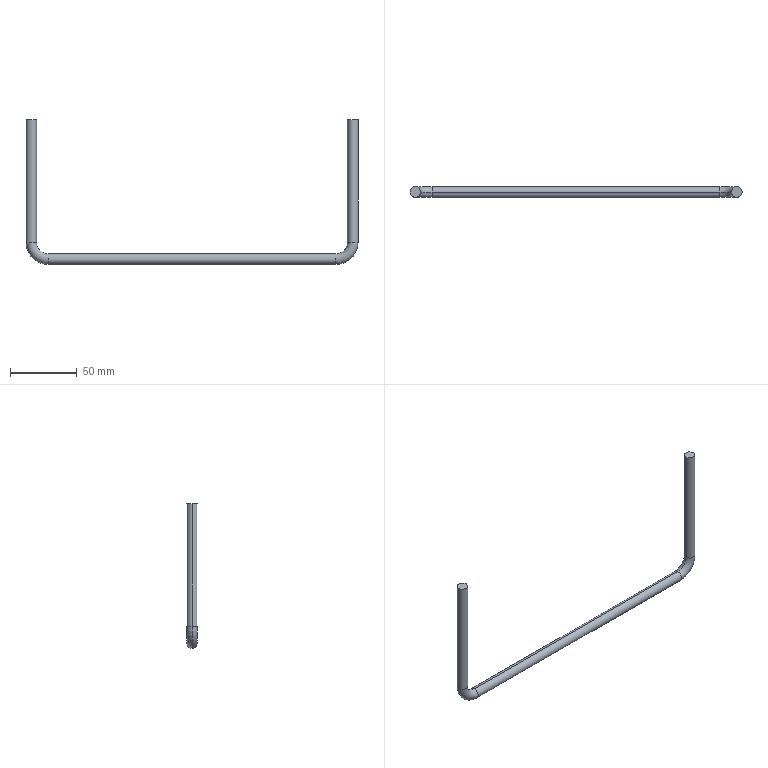Part | NX | features BREP 1 | 1 solid | 12 faces | box 249.238 x 7.938 x 108.744 mm | volume 21770 mm3 | cylinder 6 | torus 4 | plane 2 | commonest cylinder face diameters 7.938 x6
STEP:
#1=CARTESIAN_POINT('',(-116.681,0.,0.));
#2=VERTEX_POINT('',#1);
#3=CARTESIAN_POINT('',(-124.619,0.,0.));
#4=VERTEX_POINT('',#3);
#5=CARTESIAN_POINT('',(-120.65,0.,0.));
#6=DIRECTION('',(0.,0.,-1.));
#7=DIRECTION('',(1.,0.,0.));
#8=AXIS2_PLACEMENT_3D('',#5,#6,#7);
#9=CIRCLE('',#8,3.969);
#10=EDGE_CURVE('',#2,#4,#9,.T.);
#11=ORIENTED_EDGE('',*,*,#10,.F.);
#12=CARTESIAN_POINT('',(-120.65,0.,0.));
#13=DIRECTION('',(0.,0.,-1.));
#14=DIRECTION('',(-1.,0.,0.));
#15=AXIS2_PLACEMENT_3D('',#12,#13,#14);
#16=CIRCLE('',#15,3.969);
#17=EDGE_CURVE('',#4,#2,#16,.T.);
#18=ORIENTED_EDGE('',*,*,#17,.F.);
#19=EDGE_LOOP('',(#11,#18));
#20=FACE_BOUND('',#19,.T.);
#21=CARTESIAN_POINT('',(-120.65,0.,0.));
#22=DIRECTION('',(0.,0.,-1.));
#23=DIRECTION('',(0.,-1.,0.));
#24=AXIS2_PLACEMENT_3D('',#21,#22,#23);
#25=PLANE('',#24);
#26=ADVANCED_FACE('',(#20),#25,.F.);
#27=CARTESIAN_POINT('',(-116.681,0.,-92.075));
#28=VERTEX_POINT('',#27);
#29=CARTESIAN_POINT('',(-116.681,0.,0.));
#30=DIRECTION('',(0.,0.,-1.));
#31=VECTOR('',#30,1000.);
#32=LINE('',#29,#31);
#33=EDGE_CURVE('',#28,#2,#32,.F.);
#34=ORIENTED_EDGE('',*,*,#33,.F.);
#35=CARTESIAN_POINT('',(-124.619,0.,-92.075));
#36=VERTEX_POINT('',#35);
#37=CARTESIAN_POINT('',(-120.65,0.,-92.075));
#38=DIRECTION('',(0.,0.,-1.));
#39=DIRECTION('',(-1.,0.,0.));
#40=AXIS2_PLACEMENT_3D('',#37,#38,#39);
#41=CIRCLE('',#40,3.969);
#42=EDGE_CURVE('',#36,#28,#41,.T.);
#43=ORIENTED_EDGE('',*,*,#42,.F.);
#44=CARTESIAN_POINT('',(-124.619,0.,0.));
#45=DIRECTION('',(0.,0.,-1.));
#46=VECTOR('',#45,1000.);
#47=LINE('',#44,#46);
#48=EDGE_CURVE('',#36,#4,#47,.F.);
#49=ORIENTED_EDGE('',*,*,#48,.T.);
#50=ORIENTED_EDGE('',*,*,#17,.T.);
#51=EDGE_LOOP('',(#34,#43,#49,#50));
#52=FACE_BOUND('',#51,.T.);
#53=CARTESIAN_POINT('',(-120.65,0.,0.));
#54=DIRECTION('',(0.,0.,-1.));
#55=DIRECTION('',(-1.,0.,0.));
#56=AXIS2_PLACEMENT_3D('',#53,#54,#55);
#57=CYLINDRICAL_SURFACE('',#56,3.969);
#58=ADVANCED_FACE('',(#52),#57,.T.);
#59=ORIENTED_EDGE('',*,*,#48,.F.);
#60=CARTESIAN_POINT('',(-120.65,0.,-92.075));
#61=DIRECTION('',(0.,0.,-1.));
#62=DIRECTION('',(1.,0.,0.));
#63=AXIS2_PLACEMENT_3D('',#60,#61,#62);
#64=CIRCLE('',#63,3.969);
#65=EDGE_CURVE('',#28,#36,#64,.T.);
#66=ORIENTED_EDGE('',*,*,#65,.F.);
#67=ORIENTED_EDGE('',*,*,#33,.T.);
#68=ORIENTED_EDGE('',*,*,#10,.T.);
#69=EDGE_LOOP('',(#59,#66,#67,#68));
#70=FACE_BOUND('',#69,.T.);
#71=CARTESIAN_POINT('',(-120.65,0.,0.));
#72=DIRECTION('',(0.,0.,-1.));
#73=DIRECTION('',(-1.,0.,0.));
#74=AXIS2_PLACEMENT_3D('',#71,#72,#73);
#75=CYLINDRICAL_SURFACE('',#74,3.969);
#76=ADVANCED_FACE('',(#70),#75,.T.);
#77=CARTESIAN_POINT('',(-107.95,0.,-108.744));
#78=VERTEX_POINT('',#77);
#79=CARTESIAN_POINT('',(-107.95,0.,-92.075));
#80=DIRECTION('',(0.,-1.,0.));
#81=DIRECTION('',(-1.,0.,0.));
#82=AXIS2_PLACEMENT_3D('',#79,#80,#81);
#83=CIRCLE('',#82,16.669);
#84=EDGE_CURVE('',#36,#78,#83,.T.);
#85=ORIENTED_EDGE('',*,*,#84,.T.);
#86=CARTESIAN_POINT('',(-107.95,0.,-100.806));
#87=VERTEX_POINT('',#86);
#88=CARTESIAN_POINT('',(-107.95,0.,-104.775));
#89=DIRECTION('',(1.,0.,0.));
#90=DIRECTION('',(0.,0.,1.));
#91=AXIS2_PLACEMENT_3D('',#88,#89,#90);
#92=CIRCLE('',#91,3.969);
#93=EDGE_CURVE('',#87,#78,#92,.T.);
#94=ORIENTED_EDGE('',*,*,#93,.F.);
#95=CARTESIAN_POINT('',(-107.95,0.,-92.075));
#96=DIRECTION('',(0.,-1.,0.));
#97=DIRECTION('',(-1.,0.,0.));
#98=AXIS2_PLACEMENT_3D('',#95,#96,#97);
#99=CIRCLE('',#98,8.731);
#100=EDGE_CURVE('',#28,#87,#99,.T.);
#101=ORIENTED_EDGE('',*,*,#100,.F.);
#102=ORIENTED_EDGE('',*,*,#65,.T.);
#103=EDGE_LOOP('',(#85,#94,#101,#102));
#104=FACE_BOUND('',#103,.T.);
#105=CARTESIAN_POINT('',(-107.95,0.,-92.075));
#106=DIRECTION('',(0.,-1.,0.));
#107=DIRECTION('',(1.,0.,0.));
#108=AXIS2_PLACEMENT_3D('',#105,#106,#107);
#109=TOROIDAL_SURFACE('',#108,12.7,3.969);
#110=ADVANCED_FACE('',(#104),#109,.T.);
#111=ORIENTED_EDGE('',*,*,#100,.T.);
#112=CARTESIAN_POINT('',(-107.95,0.,-104.775));
#113=DIRECTION('',(1.,0.,0.));
#114=DIRECTION('',(0.,0.,-1.));
#115=AXIS2_PLACEMENT_3D('',#112,#113,#114);
#116=CIRCLE('',#115,3.969);
#117=EDGE_CURVE('',#78,#87,#116,.T.);
#118=ORIENTED_EDGE('',*,*,#117,.F.);
#119=ORIENTED_EDGE('',*,*,#84,.F.);
#120=ORIENTED_EDGE('',*,*,#42,.T.);
#121=EDGE_LOOP('',(#111,#118,#119,#120));
#122=FACE_BOUND('',#121,.T.);
#123=CARTESIAN_POINT('',(-107.95,0.,-92.075));
#124=DIRECTION('',(0.,-1.,0.));
#125=DIRECTION('',(1.,0.,0.));
#126=AXIS2_PLACEMENT_3D('',#123,#124,#125);
#127=TOROIDAL_SURFACE('',#126,12.7,3.969);
#128=ADVANCED_FACE('',(#122),#127,.T.);
#129=CARTESIAN_POINT('',(107.95,0.,-100.806));
#130=VERTEX_POINT('',#129);
#131=CARTESIAN_POINT('',(-107.95,0.,-100.806));
#132=DIRECTION('',(1.,0.,0.));
#133=VECTOR('',#132,1000.);
#134=LINE('',#131,#133);
#135=EDGE_CURVE('',#130,#87,#134,.F.);
#136=ORIENTED_EDGE('',*,*,#135,.F.);
#137=CARTESIAN_POINT('',(107.95,0.,-108.744));
#138=VERTEX_POINT('',#137);
#139=CARTESIAN_POINT('',(107.95,0.,-104.775));
#140=DIRECTION('',(1.,0.,0.));
#141=DIRECTION('',(0.,0.,-1.));
#142=AXIS2_PLACEMENT_3D('',#139,#140,#141);
#143=CIRCLE('',#142,3.969);
#144=EDGE_CURVE('',#138,#130,#143,.T.);
#145=ORIENTED_EDGE('',*,*,#144,.F.);
#146=CARTESIAN_POINT('',(-107.95,0.,-108.744));
#147=DIRECTION('',(1.,0.,0.));
#148=VECTOR('',#147,1000.);
#149=LINE('',#146,#148);
#150=EDGE_CURVE('',#138,#78,#149,.F.);
#151=ORIENTED_EDGE('',*,*,#150,.T.);
#152=ORIENTED_EDGE('',*,*,#117,.T.);
#153=EDGE_LOOP('',(#136,#145,#151,#152));
#154=FACE_BOUND('',#153,.T.);
#155=CARTESIAN_POINT('',(-107.95,0.,-104.775));
#156=DIRECTION('',(1.,0.,0.));
#157=DIRECTION('',(0.,0.,-1.));
#158=AXIS2_PLACEMENT_3D('',#155,#156,#157);
#159=CYLINDRICAL_SURFACE('',#158,3.969);
#160=ADVANCED_FACE('',(#154),#159,.T.);
#161=ORIENTED_EDGE('',*,*,#150,.F.);
#162=CARTESIAN_POINT('',(107.95,0.,-104.775));
#163=DIRECTION('',(1.,0.,0.));
#164=DIRECTION('',(0.,0.,1.));
#165=AXIS2_PLACEMENT_3D('',#162,#163,#164);
#166=CIRCLE('',#165,3.969);
#167=EDGE_CURVE('',#130,#138,#166,.T.);
#168=ORIENTED_EDGE('',*,*,#167,.F.);
#169=ORIENTED_EDGE('',*,*,#135,.T.);
#170=ORIENTED_EDGE('',*,*,#93,.T.);
#171=EDGE_LOOP('',(#161,#168,#169,#170));
#172=FACE_BOUND('',#171,.T.);
#173=CARTESIAN_POINT('',(-107.95,0.,-104.775));
#174=DIRECTION('',(1.,0.,0.));
#175=DIRECTION('',(0.,0.,-1.));
#176=AXIS2_PLACEMENT_3D('',#173,#174,#175);
#177=CYLINDRICAL_SURFACE('',#176,3.969);
#178=ADVANCED_FACE('',(#172),#177,.T.);
#179=CARTESIAN_POINT('',(124.619,0.,-92.075));
#180=VERTEX_POINT('',#179);
#181=CARTESIAN_POINT('',(107.95,0.,-92.075));
#182=DIRECTION('',(0.,-1.,0.));
#183=DIRECTION('',(0.,0.,-1.));
#184=AXIS2_PLACEMENT_3D('',#181,#182,#183);
#185=CIRCLE('',#184,16.669);
#186=EDGE_CURVE('',#138,#180,#185,.T.);
#187=ORIENTED_EDGE('',*,*,#186,.T.);
#188=CARTESIAN_POINT('',(116.681,0.,-92.075));
#189=VERTEX_POINT('',#188);
#190=CARTESIAN_POINT('',(120.65,0.,-92.075));
#191=DIRECTION('',(0.,0.,1.));
#192=DIRECTION('',(-1.,0.,0.));
#193=AXIS2_PLACEMENT_3D('',#190,#191,#192);
#194=CIRCLE('',#193,3.969);
#195=EDGE_CURVE('',#189,#180,#194,.T.);
#196=ORIENTED_EDGE('',*,*,#195,.F.);
#197=CARTESIAN_POINT('',(107.95,0.,-92.075));
#198=DIRECTION('',(0.,-1.,0.));
#199=DIRECTION('',(0.,0.,-1.));
#200=AXIS2_PLACEMENT_3D('',#197,#198,#199);
#201=CIRCLE('',#200,8.731);
#202=EDGE_CURVE('',#130,#189,#201,.T.);
#203=ORIENTED_EDGE('',*,*,#202,.F.);
#204=ORIENTED_EDGE('',*,*,#167,.T.);
#205=EDGE_LOOP('',(#187,#196,#203,#204));
#206=FACE_BOUND('',#205,.T.);
#207=CARTESIAN_POINT('',(107.95,0.,-92.075));
#208=DIRECTION('',(0.,-1.,0.));
#209=DIRECTION('',(0.,0.,1.));
#210=AXIS2_PLACEMENT_3D('',#207,#208,#209);
#211=TOROIDAL_SURFACE('',#210,12.7,3.969);
#212=ADVANCED_FACE('',(#206),#211,.T.);
#213=ORIENTED_EDGE('',*,*,#202,.T.);
#214=CARTESIAN_POINT('',(120.65,0.,-92.075));
#215=DIRECTION('',(0.,0.,1.));
#216=DIRECTION('',(1.,0.,0.));
#217=AXIS2_PLACEMENT_3D('',#214,#215,#216);
#218=CIRCLE('',#217,3.969);
#219=EDGE_CURVE('',#180,#189,#218,.T.);
#220=ORIENTED_EDGE('',*,*,#219,.F.);
#221=ORIENTED_EDGE('',*,*,#186,.F.);
#222=ORIENTED_EDGE('',*,*,#144,.T.);
#223=EDGE_LOOP('',(#213,#220,#221,#222));
#224=FACE_BOUND('',#223,.T.);
#225=CARTESIAN_POINT('',(107.95,0.,-92.075));
#226=DIRECTION('',(0.,-1.,0.));
#227=DIRECTION('',(0.,0.,1.));
#228=AXIS2_PLACEMENT_3D('',#225,#226,#227);
#229=TOROIDAL_SURFACE('',#228,12.7,3.969);
#230=ADVANCED_FACE('',(#224),#229,.T.);
#231=CARTESIAN_POINT('',(116.681,0.,0.));
#232=VERTEX_POINT('',#231);
#233=CARTESIAN_POINT('',(116.681,0.,-92.075));
#234=DIRECTION('',(0.,0.,1.));
#235=VECTOR('',#234,1000.);
#236=LINE('',#233,#235);
#237=EDGE_CURVE('',#189,#232,#236,.T.);
#238=ORIENTED_EDGE('',*,*,#237,.T.);
#239=CARTESIAN_POINT('',(124.619,0.,0.));
#240=VERTEX_POINT('',#239);
#241=CARTESIAN_POINT('',(120.65,0.,0.));
#242=DIRECTION('',(0.,0.,1.));
#243=DIRECTION('',(1.,0.,0.));
#244=AXIS2_PLACEMENT_3D('',#241,#242,#243);
#245=CIRCLE('',#244,3.969);
#246=EDGE_CURVE('',#240,#232,#245,.T.);
#247=ORIENTED_EDGE('',*,*,#246,.F.);
#248=CARTESIAN_POINT('',(124.619,0.,-92.075));
#249=DIRECTION('',(0.,0.,1.));
#250=VECTOR('',#249,1000.);
#251=LINE('',#248,#250);
#252=EDGE_CURVE('',#180,#240,#251,.T.);
#253=ORIENTED_EDGE('',*,*,#252,.F.);
#254=ORIENTED_EDGE('',*,*,#219,.T.);
#255=EDGE_LOOP('',(#238,#247,#253,#254));
#256=FACE_BOUND('',#255,.T.);
#257=CARTESIAN_POINT('',(120.65,0.,-92.075));
#258=DIRECTION('',(0.,0.,1.));
#259=DIRECTION('',(1.,0.,0.));
#260=AXIS2_PLACEMENT_3D('',#257,#258,#259);
#261=CYLINDRICAL_SURFACE('',#260,3.969);
#262=ADVANCED_FACE('',(#256),#261,.T.);
#263=ORIENTED_EDGE('',*,*,#252,.T.);
#264=CARTESIAN_POINT('',(120.65,0.,0.));
#265=DIRECTION('',(0.,0.,1.));
#266=DIRECTION('',(-1.,0.,0.));
#267=AXIS2_PLACEMENT_3D('',#264,#265,#266);
#268=CIRCLE('',#267,3.969);
#269=EDGE_CURVE('',#232,#240,#268,.T.);
#270=ORIENTED_EDGE('',*,*,#269,.F.);
#271=ORIENTED_EDGE('',*,*,#237,.F.);
#272=ORIENTED_EDGE('',*,*,#195,.T.);
#273=EDGE_LOOP('',(#263,#270,#271,#272));
#274=FACE_BOUND('',#273,.T.);
#275=CARTESIAN_POINT('',(120.65,0.,-92.075));
#276=DIRECTION('',(0.,0.,1.));
#277=DIRECTION('',(1.,0.,0.));
#278=AXIS2_PLACEMENT_3D('',#275,#276,#277);
#279=CYLINDRICAL_SURFACE('',#278,3.969);
#280=ADVANCED_FACE('',(#274),#279,.T.);
#281=ORIENTED_EDGE('',*,*,#269,.T.);
#282=ORIENTED_EDGE('',*,*,#246,.T.);
#283=EDGE_LOOP('',(#281,#282));
#284=FACE_BOUND('',#283,.T.);
#285=CARTESIAN_POINT('',(120.65,0.,0.));
#286=DIRECTION('',(0.,0.,1.));
#287=DIRECTION('',(1.,0.,0.));
#288=AXIS2_PLACEMENT_3D('',#285,#286,#287);
#289=PLANE('',#288);
#290=ADVANCED_FACE('',(#284),#289,.T.);
#291=CLOSED_SHELL('',(#26,#58,#76,#110,#128,#160,#178,#212,#230,#262,#280,#290));
#292=MANIFOLD_SOLID_BREP('',#291);
#293=(LENGTH_UNIT()NAMED_UNIT(*)SI_UNIT(.MILLI.,.METRE.));
#294=UNCERTAINTY_MEASURE_WITH_UNIT(LENGTH_MEASURE(0.00001),#293,'','');
#295=(NAMED_UNIT(*)PLANE_ANGLE_UNIT()SI_UNIT($,.RADIAN.));
#296=(NAMED_UNIT(*)SI_UNIT($,.STERADIAN.)SOLID_ANGLE_UNIT());
#297=(GEOMETRIC_REPRESENTATION_CONTEXT(3)GLOBAL_UNCERTAINTY_ASSIGNED_CONTEXT((#294))GLOBAL_UNIT_ASSIGNED_CONTEXT((#293,#295,#296))REPRESENTATION_CONTEXT('',''));
#298=ADVANCED_BREP_SHAPE_REPRESENTATION('',(#292),#297);